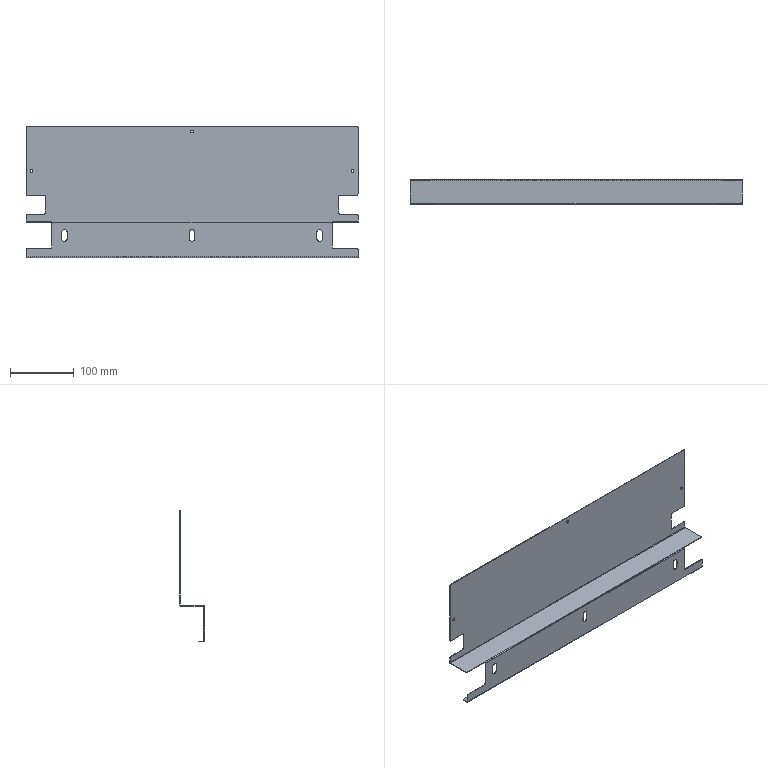Part | STEP file | Button cover plate | 1 solid | 83 faces | box 519 x 39.5 x 206 mm | volume 125183 mm3 | plane 44 | cylinder 39 | commonest cylinder face diameters 4 x18 8.5 x9 4.5 x6 1.2 x3 3.2 x3